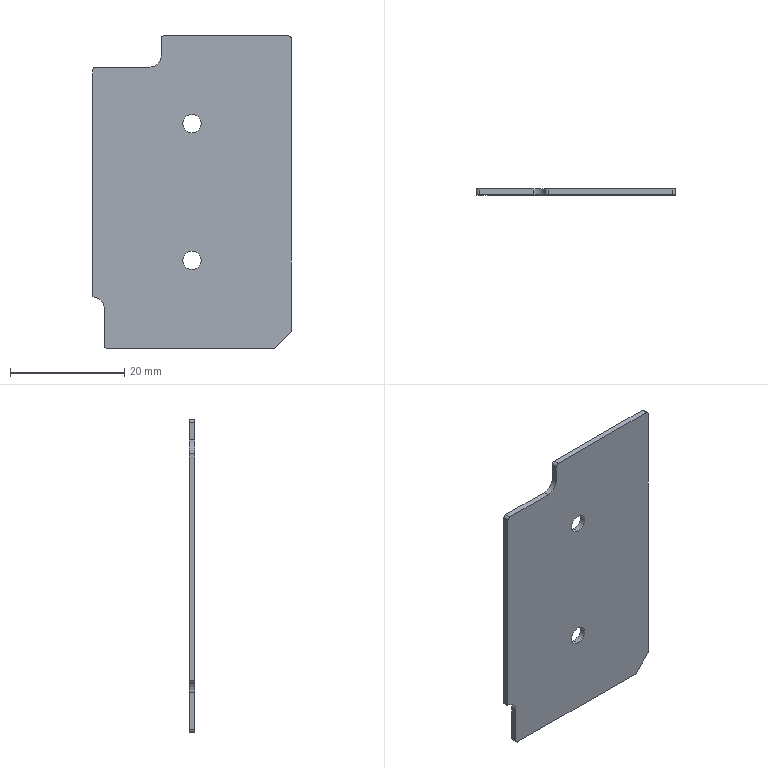Part | STEP file | Guide rail right end cap | 1 solid | 20 faces | box 34.8 x 1 x 54.8 mm | volume 1804 mm3 | cylinder 10 | plane 10 | commonest cylinder face diameters 1 x4 3.2 x4 4 x2